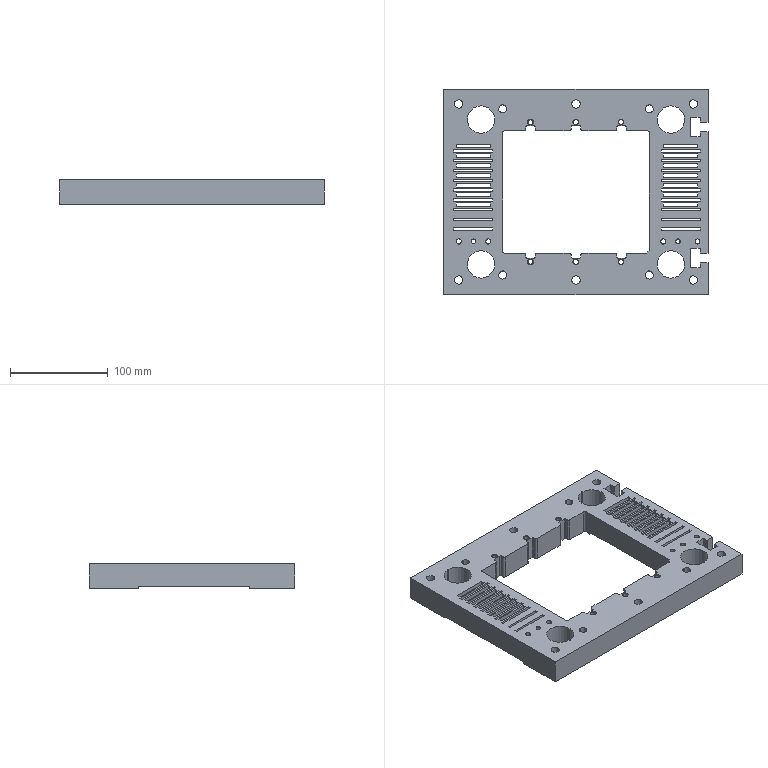Part | STEP file | 1 solid | 308 faces | box 270 x 210 x 25 mm | volume 722658 mm3 | plane 194 | cylinder 95 | cone 19 | commonest cylinder face diameters 1 x36 2.03 x12 3.97 x12 5 x6 8.6 x6 14 x6